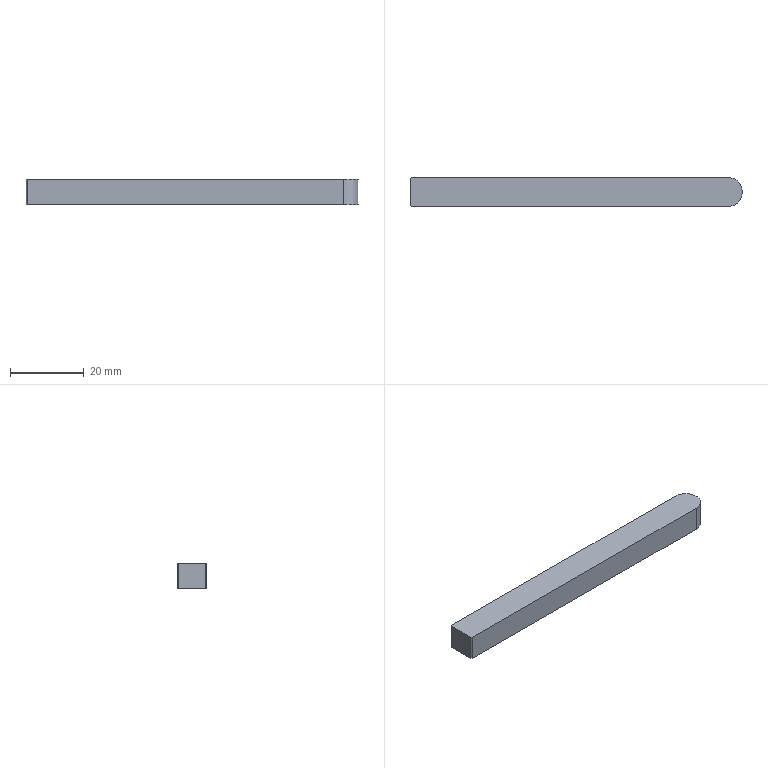Part | SolidWorks | features MBimport 1 | 1 solid | 8 faces | box 90 x 8 x 7 mm | volume 4991 mm3 | plane 7 | cylinder 1 | commonest cylinder face diameters 8 x1
STEP:
#1=CARTESIAN_POINT('',(41.,4.,0.));
#2=VERTEX_POINT('',#1);
#3=CARTESIAN_POINT('',(-44.7,4.,0.));
#4=VERTEX_POINT('',#3);
#5=CARTESIAN_POINT('',(41.,4.,0.));
#6=DIRECTION('',(-1.,0.,0.));
#7=VECTOR('',#6,1000.);
#8=LINE('',#5,#7);
#9=EDGE_CURVE('',#2,#4,#8,.T.);
#10=ORIENTED_EDGE('',*,*,#9,.T.);
#11=CARTESIAN_POINT('',(-44.7,4.,7.));
#12=VERTEX_POINT('',#11);
#13=CARTESIAN_POINT('',(-44.7,4.,7.));
#14=DIRECTION('',(0.,0.,-1.));
#15=VECTOR('',#14,1000.);
#16=LINE('',#13,#15);
#17=EDGE_CURVE('',#12,#4,#16,.T.);
#18=ORIENTED_EDGE('',*,*,#17,.F.);
#19=CARTESIAN_POINT('',(41.,4.,7.));
#20=VERTEX_POINT('',#19);
#21=CARTESIAN_POINT('',(41.,4.,7.));
#22=DIRECTION('',(-1.,0.,0.));
#23=VECTOR('',#22,1000.);
#24=LINE('',#21,#23);
#25=EDGE_CURVE('',#20,#12,#24,.T.);
#26=ORIENTED_EDGE('',*,*,#25,.F.);
#27=CARTESIAN_POINT('',(41.,4.,7.));
#28=DIRECTION('',(0.,0.,-1.));
#29=VECTOR('',#28,1000.);
#30=LINE('',#27,#29);
#31=EDGE_CURVE('',#20,#2,#30,.T.);
#32=ORIENTED_EDGE('',*,*,#31,.T.);
#33=EDGE_LOOP('',(#10,#18,#26,#32));
#34=FACE_OUTER_BOUND('',#33,.T.);
#35=CARTESIAN_POINT('',(41.,4.,7.));
#36=DIRECTION('',(0.,-1.,0.));
#37=DIRECTION('',(0.,0.,-1.));
#38=AXIS2_PLACEMENT_3D('',#35,#36,#37);
#39=PLANE('',#38);
#40=ADVANCED_FACE('',(#34),#39,.F.);
#41=CARTESIAN_POINT('',(-45.,3.7,7.));
#42=VERTEX_POINT('',#41);
#43=CARTESIAN_POINT('',(-44.7,4.,7.));
#44=DIRECTION('',(-0.7071,-0.7071,0.));
#45=VECTOR('',#44,1000.);
#46=LINE('',#43,#45);
#47=EDGE_CURVE('',#12,#42,#46,.T.);
#48=ORIENTED_EDGE('',*,*,#47,.T.);
#49=CARTESIAN_POINT('',(-45.,-3.7,7.));
#50=VERTEX_POINT('',#49);
#51=CARTESIAN_POINT('',(-45.,3.7,7.));
#52=DIRECTION('',(0.,-1.,0.));
#53=VECTOR('',#52,1000.);
#54=LINE('',#51,#53);
#55=EDGE_CURVE('',#42,#50,#54,.T.);
#56=ORIENTED_EDGE('',*,*,#55,.T.);
#57=CARTESIAN_POINT('',(-44.7,-4.,7.));
#58=VERTEX_POINT('',#57);
#59=CARTESIAN_POINT('',(-45.,-3.7,7.));
#60=DIRECTION('',(0.7071,-0.7071,0.));
#61=VECTOR('',#60,1000.);
#62=LINE('',#59,#61);
#63=EDGE_CURVE('',#50,#58,#62,.T.);
#64=ORIENTED_EDGE('',*,*,#63,.T.);
#65=CARTESIAN_POINT('',(41.,-4.,7.));
#66=VERTEX_POINT('',#65);
#67=CARTESIAN_POINT('',(-44.7,-4.,7.));
#68=DIRECTION('',(1.,0.,0.));
#69=VECTOR('',#68,1000.);
#70=LINE('',#67,#69);
#71=EDGE_CURVE('',#58,#66,#70,.T.);
#72=ORIENTED_EDGE('',*,*,#71,.T.);
#73=CARTESIAN_POINT('',(41.,0.,7.));
#74=DIRECTION('',(0.,0.,1.));
#75=DIRECTION('',(1.,0.,0.));
#76=AXIS2_PLACEMENT_3D('',#73,#74,#75);
#77=CIRCLE('',#76,4.);
#78=EDGE_CURVE('',#66,#20,#77,.T.);
#79=ORIENTED_EDGE('',*,*,#78,.T.);
#80=ORIENTED_EDGE('',*,*,#25,.T.);
#81=EDGE_LOOP('',(#48,#56,#64,#72,#79,#80));
#82=FACE_OUTER_BOUND('',#81,.T.);
#83=CARTESIAN_POINT('',(41.,0.,7.));
#84=DIRECTION('',(0.,0.,1.));
#85=DIRECTION('',(1.,0.,0.));
#86=AXIS2_PLACEMENT_3D('',#83,#84,#85);
#87=PLANE('',#86);
#88=ADVANCED_FACE('',(#82),#87,.T.);
#89=CARTESIAN_POINT('',(41.,-4.,0.));
#90=VERTEX_POINT('',#89);
#91=CARTESIAN_POINT('',(41.,0.,0.));
#92=DIRECTION('',(0.,0.,1.));
#93=DIRECTION('',(1.,0.,0.));
#94=AXIS2_PLACEMENT_3D('',#91,#92,#93);
#95=CIRCLE('',#94,4.);
#96=EDGE_CURVE('',#90,#2,#95,.T.);
#97=ORIENTED_EDGE('',*,*,#96,.T.);
#98=ORIENTED_EDGE('',*,*,#31,.F.);
#99=ORIENTED_EDGE('',*,*,#78,.F.);
#100=CARTESIAN_POINT('',(41.,-4.,7.));
#101=DIRECTION('',(0.,0.,-1.));
#102=VECTOR('',#101,1000.);
#103=LINE('',#100,#102);
#104=EDGE_CURVE('',#66,#90,#103,.T.);
#105=ORIENTED_EDGE('',*,*,#104,.T.);
#106=EDGE_LOOP('',(#97,#98,#99,#105));
#107=FACE_OUTER_BOUND('',#106,.T.);
#108=CARTESIAN_POINT('',(41.,0.,7.));
#109=DIRECTION('',(0.,0.,1.));
#110=DIRECTION('',(-1.,0.,0.));
#111=AXIS2_PLACEMENT_3D('',#108,#109,#110);
#112=CYLINDRICAL_SURFACE('',#111,4.);
#113=ADVANCED_FACE('',(#107),#112,.T.);
#114=CARTESIAN_POINT('',(-45.,3.7,0.));
#115=VERTEX_POINT('',#114);
#116=CARTESIAN_POINT('',(-44.7,4.,0.));
#117=DIRECTION('',(-0.7071,-0.7071,0.));
#118=VECTOR('',#117,1000.);
#119=LINE('',#116,#118);
#120=EDGE_CURVE('',#4,#115,#119,.T.);
#121=ORIENTED_EDGE('',*,*,#120,.T.);
#122=CARTESIAN_POINT('',(-45.,3.7,7.));
#123=DIRECTION('',(0.,0.,-1.));
#124=VECTOR('',#123,1000.);
#125=LINE('',#122,#124);
#126=EDGE_CURVE('',#42,#115,#125,.T.);
#127=ORIENTED_EDGE('',*,*,#126,.F.);
#128=ORIENTED_EDGE('',*,*,#47,.F.);
#129=ORIENTED_EDGE('',*,*,#17,.T.);
#130=EDGE_LOOP('',(#121,#127,#128,#129));
#131=FACE_OUTER_BOUND('',#130,.T.);
#132=CARTESIAN_POINT('',(-44.7,4.,7.));
#133=DIRECTION('',(0.7071,-0.7071,0.));
#134=DIRECTION('',(0.,0.,-1.));
#135=AXIS2_PLACEMENT_3D('',#132,#133,#134);
#136=PLANE('',#135);
#137=ADVANCED_FACE('',(#131),#136,.F.);
#138=CARTESIAN_POINT('',(-45.,-3.7,0.));
#139=VERTEX_POINT('',#138);
#140=CARTESIAN_POINT('',(-45.,3.7,0.));
#141=DIRECTION('',(0.,-1.,0.));
#142=VECTOR('',#141,1000.);
#143=LINE('',#140,#142);
#144=EDGE_CURVE('',#115,#139,#143,.T.);
#145=ORIENTED_EDGE('',*,*,#144,.T.);
#146=CARTESIAN_POINT('',(-45.,-3.7,7.));
#147=DIRECTION('',(0.,0.,-1.));
#148=VECTOR('',#147,1000.);
#149=LINE('',#146,#148);
#150=EDGE_CURVE('',#50,#139,#149,.T.);
#151=ORIENTED_EDGE('',*,*,#150,.F.);
#152=ORIENTED_EDGE('',*,*,#55,.F.);
#153=ORIENTED_EDGE('',*,*,#126,.T.);
#154=EDGE_LOOP('',(#145,#151,#152,#153));
#155=FACE_OUTER_BOUND('',#154,.T.);
#156=CARTESIAN_POINT('',(-45.,3.7,7.));
#157=DIRECTION('',(1.,0.,0.));
#158=DIRECTION('',(0.,1.,0.));
#159=AXIS2_PLACEMENT_3D('',#156,#157,#158);
#160=PLANE('',#159);
#161=ADVANCED_FACE('',(#155),#160,.F.);
#162=CARTESIAN_POINT('',(-44.7,-4.,0.));
#163=VERTEX_POINT('',#162);
#164=CARTESIAN_POINT('',(-45.,-3.7,0.));
#165=DIRECTION('',(0.7071,-0.7071,0.));
#166=VECTOR('',#165,1000.);
#167=LINE('',#164,#166);
#168=EDGE_CURVE('',#139,#163,#167,.T.);
#169=ORIENTED_EDGE('',*,*,#168,.T.);
#170=CARTESIAN_POINT('',(-44.7,-4.,7.));
#171=DIRECTION('',(0.,0.,-1.));
#172=VECTOR('',#171,1000.);
#173=LINE('',#170,#172);
#174=EDGE_CURVE('',#58,#163,#173,.T.);
#175=ORIENTED_EDGE('',*,*,#174,.F.);
#176=ORIENTED_EDGE('',*,*,#63,.F.);
#177=ORIENTED_EDGE('',*,*,#150,.T.);
#178=EDGE_LOOP('',(#169,#175,#176,#177));
#179=FACE_OUTER_BOUND('',#178,.T.);
#180=CARTESIAN_POINT('',(-45.,-3.7,7.));
#181=DIRECTION('',(0.7071,0.7071,0.));
#182=DIRECTION('',(0.,0.,-1.));
#183=AXIS2_PLACEMENT_3D('',#180,#181,#182);
#184=PLANE('',#183);
#185=ADVANCED_FACE('',(#179),#184,.F.);
#186=CARTESIAN_POINT('',(-44.7,-4.,0.));
#187=DIRECTION('',(1.,0.,0.));
#188=VECTOR('',#187,1000.);
#189=LINE('',#186,#188);
#190=EDGE_CURVE('',#163,#90,#189,.T.);
#191=ORIENTED_EDGE('',*,*,#190,.T.);
#192=ORIENTED_EDGE('',*,*,#104,.F.);
#193=ORIENTED_EDGE('',*,*,#71,.F.);
#194=ORIENTED_EDGE('',*,*,#174,.T.);
#195=EDGE_LOOP('',(#191,#192,#193,#194));
#196=FACE_OUTER_BOUND('',#195,.T.);
#197=CARTESIAN_POINT('',(-44.7,-4.,7.));
#198=DIRECTION('',(0.,1.,0.));
#199=DIRECTION('',(1.,0.,0.));
#200=AXIS2_PLACEMENT_3D('',#197,#198,#199);
#201=PLANE('',#200);
#202=ADVANCED_FACE('',(#196),#201,.F.);
#203=ORIENTED_EDGE('',*,*,#120,.F.);
#204=ORIENTED_EDGE('',*,*,#9,.F.);
#205=ORIENTED_EDGE('',*,*,#96,.F.);
#206=ORIENTED_EDGE('',*,*,#190,.F.);
#207=ORIENTED_EDGE('',*,*,#168,.F.);
#208=ORIENTED_EDGE('',*,*,#144,.F.);
#209=EDGE_LOOP('',(#203,#204,#205,#206,#207,#208));
#210=FACE_OUTER_BOUND('',#209,.T.);
#211=CARTESIAN_POINT('',(41.,0.,0.));
#212=DIRECTION('',(0.,0.,1.));
#213=DIRECTION('',(1.,0.,0.));
#214=AXIS2_PLACEMENT_3D('',#211,#212,#213);
#215=PLANE('',#214);
#216=ADVANCED_FACE('',(#210),#215,.F.);
#217=CLOSED_SHELL('',(#40,#88,#113,#137,#161,#185,#202,#216));
#218=MANIFOLD_SOLID_BREP('',#217);
#219=CARTESIAN_POINT('',(0.,0.,0.));
#220=DIRECTION('',(0.,0.,1.));
#221=DIRECTION('',(1.,0.,0.));
#222=AXIS2_PLACEMENT_3D('',#219,#220,#221);
#223=(LENGTH_UNIT()NAMED_UNIT(*)SI_UNIT(.MILLI.,.METRE.));
#224=UNCERTAINTY_MEASURE_WITH_UNIT(LENGTH_MEASURE(0.00001),#223,'','');
#225=(NAMED_UNIT(*)PLANE_ANGLE_UNIT()SI_UNIT($,.RADIAN.));
#226=(NAMED_UNIT(*)SI_UNIT($,.STERADIAN.)SOLID_ANGLE_UNIT());
#227=(GEOMETRIC_REPRESENTATION_CONTEXT(3)GLOBAL_UNCERTAINTY_ASSIGNED_CONTEXT((#224))GLOBAL_UNIT_ASSIGNED_CONTEXT((#223,#225,#226))REPRESENTATION_CONTEXT('',''));
#228=ADVANCED_BREP_SHAPE_REPRESENTATION('',(#218,#222),#227);